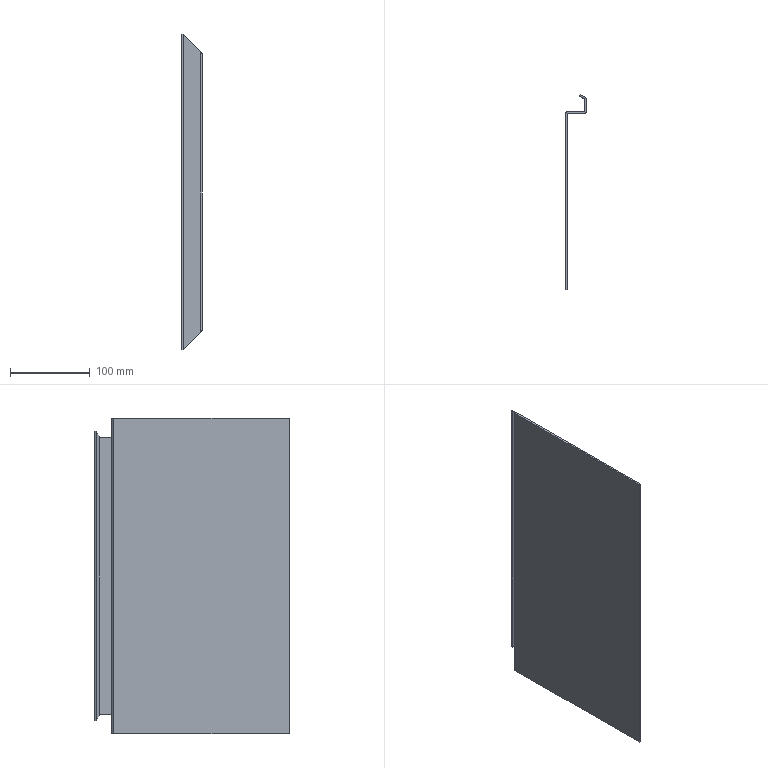Part | SolidWorks | features Cut 2, FlatPattern 1, SMBaseFlange 1, SheetMetal 1 | 1 solid | 32 faces | box 26 x 244.5 x 396 mm | volume 210973 mm3 | plane 22 | cylinder 6 | spline 4 | commonest cylinder face diameters 0.6 x3 4.6 x3
STEP:
#1=CARTESIAN_POINT('',(22.85,240.664,22.85));
#2=VERTEX_POINT('',#1);
#3=CARTESIAN_POINT('',(16.206,244.5,16.206));
#4=VERTEX_POINT('',#3);
#5=CARTESIAN_POINT('',(183.429,147.954,183.429));
#6=DIRECTION('',(-0.6547,0.378,-0.6547));
#7=VECTOR('',#6,1000.);
#8=LINE('',#5,#7);
#9=EDGE_CURVE('',#2,#4,#8,.T.);
#10=ORIENTED_EDGE('',*,*,#9,.T.);
#11=CARTESIAN_POINT('',(16.206,244.5,379.794));
#12=VERTEX_POINT('',#11);
#13=CARTESIAN_POINT('',(16.206,244.5,396.));
#14=DIRECTION('',(0.,0.,-1.));
#15=VECTOR('',#14,1000.);
#16=LINE('',#13,#15);
#17=EDGE_CURVE('',#12,#4,#16,.T.);
#18=ORIENTED_EDGE('',*,*,#17,.F.);
#19=CARTESIAN_POINT('',(22.85,240.664,373.15));
#20=VERTEX_POINT('',#19);
#21=CARTESIAN_POINT('',(13.714,245.938,382.286));
#22=DIRECTION('',(0.6547,-0.378,-0.6547));
#23=VECTOR('',#22,1000.);
#24=LINE('',#21,#23);
#25=EDGE_CURVE('',#12,#20,#24,.T.);
#26=ORIENTED_EDGE('',*,*,#25,.T.);
#27=CARTESIAN_POINT('',(22.85,240.664,396.));
#28=DIRECTION('',(0.,0.,-1.));
#29=VECTOR('',#28,1000.);
#30=LINE('',#27,#29);
#31=EDGE_CURVE('',#20,#2,#30,.T.);
#32=ORIENTED_EDGE('',*,*,#31,.T.);
#33=EDGE_LOOP('',(#10,#18,#26,#32));
#34=FACE_OUTER_BOUND('',#33,.T.);
#35=CARTESIAN_POINT('',(24.,240.,396.));
#36=DIRECTION('',(-0.5,-0.866,0.));
#37=DIRECTION('',(0.866,-0.5,0.));
#38=AXIS2_PLACEMENT_3D('',#35,#36,#37);
#39=PLANE('',#38);
#40=ADVANCED_FACE('',(#34),#39,.F.);
#41=ORIENTED_EDGE('',*,*,#17,.T.);
#42=CARTESIAN_POINT('',(15.206,242.768,16.206));
#43=VERTEX_POINT('',#42);
#44=CARTESIAN_POINT('',(16.206,244.5,16.206));
#45=DIRECTION('',(-0.5,-0.866,0.));
#46=VECTOR('',#45,1000.);
#47=LINE('',#44,#46);
#48=EDGE_CURVE('',#4,#43,#47,.T.);
#49=ORIENTED_EDGE('',*,*,#48,.T.);
#50=CARTESIAN_POINT('',(15.206,242.768,379.794));
#51=VERTEX_POINT('',#50);
#52=CARTESIAN_POINT('',(15.206,242.768,396.));
#53=DIRECTION('',(0.,0.,-1.));
#54=VECTOR('',#53,1000.);
#55=LINE('',#52,#54);
#56=EDGE_CURVE('',#51,#43,#55,.T.);
#57=ORIENTED_EDGE('',*,*,#56,.F.);
#58=CARTESIAN_POINT('',(16.206,244.5,379.794));
#59=DIRECTION('',(-0.5,-0.866,0.));
#60=VECTOR('',#59,1000.);
#61=LINE('',#58,#60);
#62=EDGE_CURVE('',#12,#51,#61,.T.);
#63=ORIENTED_EDGE('',*,*,#62,.F.);
#64=EDGE_LOOP('',(#41,#49,#57,#63));
#65=FACE_OUTER_BOUND('',#64,.T.);
#66=CARTESIAN_POINT('',(15.206,242.768,396.));
#67=DIRECTION('',(-0.866,0.5,0.));
#68=DIRECTION('',(-0.5,-0.866,0.));
#69=AXIS2_PLACEMENT_3D('',#66,#67,#68);
#70=PLANE('',#69);
#71=ADVANCED_FACE('',(#65),#70,.T.);
#72=ORIENTED_EDGE('',*,*,#56,.T.);
#73=CARTESIAN_POINT('',(21.85,238.932,22.85));
#74=VERTEX_POINT('',#73);
#75=CARTESIAN_POINT('',(182.429,146.222,183.429));
#76=DIRECTION('',(-0.6547,0.378,-0.6547));
#77=VECTOR('',#76,1000.);
#78=LINE('',#75,#77);
#79=EDGE_CURVE('',#74,#43,#78,.T.);
#80=ORIENTED_EDGE('',*,*,#79,.F.);
#81=CARTESIAN_POINT('',(21.85,238.932,373.15));
#82=VERTEX_POINT('',#81);
#83=CARTESIAN_POINT('',(21.85,238.932,396.));
#84=DIRECTION('',(0.,0.,-1.));
#85=VECTOR('',#84,1000.);
#86=LINE('',#83,#85);
#87=EDGE_CURVE('',#82,#74,#86,.T.);
#88=ORIENTED_EDGE('',*,*,#87,.F.);
#89=CARTESIAN_POINT('',(12.714,244.206,382.286));
#90=DIRECTION('',(0.6547,-0.378,-0.6547));
#91=VECTOR('',#90,1000.);
#92=LINE('',#89,#91);
#93=EDGE_CURVE('',#51,#82,#92,.T.);
#94=ORIENTED_EDGE('',*,*,#93,.F.);
#95=EDGE_LOOP('',(#72,#80,#88,#94));
#96=FACE_OUTER_BOUND('',#95,.T.);
#97=CARTESIAN_POINT('',(23.,238.268,396.));
#98=DIRECTION('',(-0.5,-0.866,0.));
#99=DIRECTION('',(0.866,-0.5,0.));
#100=AXIS2_PLACEMENT_3D('',#97,#98,#99);
#101=PLANE('',#100);
#102=ADVANCED_FACE('',(#96),#101,.T.);
#103=ORIENTED_EDGE('',*,*,#87,.T.);
#104=CARTESIAN_POINT('',(22.,238.672,24.));
#105=VERTEX_POINT('',#104);
#106=CARTESIAN_POINT('',(22.,238.672,24.));
#107=CARTESIAN_POINT('',(22.,238.782,24.));
#108=CARTESIAN_POINT('',(21.945,238.877,23.579));
#109=CARTESIAN_POINT('',(21.85,238.932,22.85));
#110=(BOUNDED_CURVE()B_SPLINE_CURVE(3,(#106,#107,#108,#109),.UNSPECIFIED.,.F.,.F.)B_SPLINE_CURVE_WITH_KNOTS((4,4),(3.142,4.189),.UNSPECIFIED.)CURVE()GEOMETRIC_REPRESENTATION_ITEM()RATIONAL_B_SPLINE_CURVE((1.,0.9107,0.9107,1.))REPRESENTATION_ITEM(''));
#111=EDGE_CURVE('',#105,#74,#110,.T.);
#112=ORIENTED_EDGE('',*,*,#111,.F.);
#113=CARTESIAN_POINT('',(22.,238.672,372.));
#114=VERTEX_POINT('',#113);
#115=CARTESIAN_POINT('',(22.,238.672,396.));
#116=DIRECTION('',(0.,0.,-1.));
#117=VECTOR('',#116,1000.);
#118=LINE('',#115,#117);
#119=EDGE_CURVE('',#114,#105,#118,.T.);
#120=ORIENTED_EDGE('',*,*,#119,.F.);
#121=CARTESIAN_POINT('',(21.85,238.932,373.15));
#122=CARTESIAN_POINT('',(21.945,238.877,372.421));
#123=CARTESIAN_POINT('',(22.,238.782,372.));
#124=CARTESIAN_POINT('',(22.,238.672,372.));
#125=(BOUNDED_CURVE()B_SPLINE_CURVE(3,(#121,#122,#123,#124),.UNSPECIFIED.,.F.,.F.)B_SPLINE_CURVE_WITH_KNOTS((4,4),(5.236,6.283),.UNSPECIFIED.)CURVE()GEOMETRIC_REPRESENTATION_ITEM()RATIONAL_B_SPLINE_CURVE((1.,0.9107,0.9107,1.))REPRESENTATION_ITEM(''));
#126=EDGE_CURVE('',#82,#114,#125,.T.);
#127=ORIENTED_EDGE('',*,*,#126,.F.);
#128=EDGE_LOOP('',(#103,#112,#120,#127));
#129=FACE_OUTER_BOUND('',#128,.T.);
#130=CARTESIAN_POINT('',(21.7,238.672,396.));
#131=DIRECTION('',(0.,0.,-1.));
#132=DIRECTION('',(-1.,0.,0.));
#133=AXIS2_PLACEMENT_3D('',#130,#131,#132);
#134=CYLINDRICAL_SURFACE('',#133,0.3);
#135=ADVANCED_FACE('',(#129),#134,.F.);
#136=ORIENTED_EDGE('',*,*,#119,.T.);
#137=CARTESIAN_POINT('',(22.,223.3,24.));
#138=VERTEX_POINT('',#137);
#139=CARTESIAN_POINT('',(22.,221.,24.));
#140=DIRECTION('',(0.,1.,0.));
#141=VECTOR('',#140,1000.);
#142=LINE('',#139,#141);
#143=EDGE_CURVE('',#138,#105,#142,.T.);
#144=ORIENTED_EDGE('',*,*,#143,.F.);
#145=CARTESIAN_POINT('',(22.,223.3,372.));
#146=VERTEX_POINT('',#145);
#147=CARTESIAN_POINT('',(22.,223.3,396.));
#148=DIRECTION('',(0.,0.,-1.));
#149=VECTOR('',#148,1000.);
#150=LINE('',#147,#149);
#151=EDGE_CURVE('',#146,#138,#150,.T.);
#152=ORIENTED_EDGE('',*,*,#151,.F.);
#153=CARTESIAN_POINT('',(22.,221.,372.));
#154=DIRECTION('',(0.,-1.,0.));
#155=VECTOR('',#154,1000.);
#156=LINE('',#153,#155);
#157=EDGE_CURVE('',#114,#146,#156,.T.);
#158=ORIENTED_EDGE('',*,*,#157,.F.);
#159=EDGE_LOOP('',(#136,#144,#152,#158));
#160=FACE_OUTER_BOUND('',#159,.T.);
#161=CARTESIAN_POINT('',(22.,221.,396.));
#162=DIRECTION('',(-1.,0.,0.));
#163=DIRECTION('',(0.,0.,1.));
#164=AXIS2_PLACEMENT_3D('',#161,#162,#163);
#165=PLANE('',#164);
#166=ADVANCED_FACE('',(#160),#165,.T.);
#167=ORIENTED_EDGE('',*,*,#151,.T.);
#168=CARTESIAN_POINT('',(21.7,223.,21.7));
#169=VERTEX_POINT('',#168);
#170=CARTESIAN_POINT('',(21.7,223.,21.7));
#171=CARTESIAN_POINT('',(21.876,223.,23.047));
#172=CARTESIAN_POINT('',(22.,223.124,24.));
#173=CARTESIAN_POINT('',(22.,223.3,24.));
#174=(BOUNDED_CURVE()B_SPLINE_CURVE(3,(#170,#171,#172,#173),.UNSPECIFIED.,.F.,.F.)B_SPLINE_CURVE_WITH_KNOTS((4,4),(1.571,3.142),.UNSPECIFIED.)CURVE()GEOMETRIC_REPRESENTATION_ITEM()RATIONAL_B_SPLINE_CURVE((1.,0.8047,0.8047,1.))REPRESENTATION_ITEM(''));
#175=EDGE_CURVE('',#169,#138,#174,.T.);
#176=ORIENTED_EDGE('',*,*,#175,.F.);
#177=CARTESIAN_POINT('',(21.7,223.,374.3));
#178=VERTEX_POINT('',#177);
#179=CARTESIAN_POINT('',(21.7,223.,396.));
#180=DIRECTION('',(0.,0.,-1.));
#181=VECTOR('',#180,1000.);
#182=LINE('',#179,#181);
#183=EDGE_CURVE('',#178,#169,#182,.T.);
#184=ORIENTED_EDGE('',*,*,#183,.F.);
#185=CARTESIAN_POINT('',(22.,223.3,372.));
#186=CARTESIAN_POINT('',(22.,223.124,372.));
#187=CARTESIAN_POINT('',(21.876,223.,372.953));
#188=CARTESIAN_POINT('',(21.7,223.,374.3));
#189=(BOUNDED_CURVE()B_SPLINE_CURVE(3,(#185,#186,#187,#188),.UNSPECIFIED.,.F.,.F.)B_SPLINE_CURVE_WITH_KNOTS((4,4),(0.,1.571),.UNSPECIFIED.)CURVE()GEOMETRIC_REPRESENTATION_ITEM()RATIONAL_B_SPLINE_CURVE((1.,0.8047,0.8047,1.))REPRESENTATION_ITEM(''));
#190=EDGE_CURVE('',#146,#178,#189,.T.);
#191=ORIENTED_EDGE('',*,*,#190,.F.);
#192=EDGE_LOOP('',(#167,#176,#184,#191));
#193=FACE_OUTER_BOUND('',#192,.T.);
#194=CARTESIAN_POINT('',(21.7,223.3,396.));
#195=DIRECTION('',(0.,0.,-1.));
#196=DIRECTION('',(-1.,0.,0.));
#197=AXIS2_PLACEMENT_3D('',#194,#195,#196);
#198=CYLINDRICAL_SURFACE('',#197,0.3);
#199=ADVANCED_FACE('',(#193),#198,.F.);
#200=ORIENTED_EDGE('',*,*,#183,.T.);
#201=CARTESIAN_POINT('',(0.3,223.,0.3));
#202=VERTEX_POINT('',#201);
#203=CARTESIAN_POINT('',(198.,223.,198.));
#204=DIRECTION('',(0.7071,0.,0.7071));
#205=VECTOR('',#204,1000.);
#206=LINE('',#203,#205);
#207=EDGE_CURVE('',#202,#169,#206,.T.);
#208=ORIENTED_EDGE('',*,*,#207,.F.);
#209=CARTESIAN_POINT('',(0.3,223.,395.7));
#210=VERTEX_POINT('',#209);
#211=CARTESIAN_POINT('',(0.3,223.,396.));
#212=DIRECTION('',(0.,0.,-1.));
#213=VECTOR('',#212,1000.);
#214=LINE('',#211,#213);
#215=EDGE_CURVE('',#210,#202,#214,.T.);
#216=ORIENTED_EDGE('',*,*,#215,.F.);
#217=CARTESIAN_POINT('',(0.,223.,396.));
#218=DIRECTION('',(-0.7071,0.,0.7071));
#219=VECTOR('',#218,1000.);
#220=LINE('',#217,#219);
#221=EDGE_CURVE('',#178,#210,#220,.T.);
#222=ORIENTED_EDGE('',*,*,#221,.F.);
#223=EDGE_LOOP('',(#200,#208,#216,#222));
#224=FACE_OUTER_BOUND('',#223,.T.);
#225=CARTESIAN_POINT('',(0.,223.,396.));
#226=DIRECTION('',(0.,1.,0.));
#227=DIRECTION('',(0.,0.,1.));
#228=AXIS2_PLACEMENT_3D('',#225,#226,#227);
#229=PLANE('',#228);
#230=ADVANCED_FACE('',(#224),#229,.T.);
#231=CARTESIAN_POINT('',(0.3,221.,0.3));
#232=VERTEX_POINT('',#231);
#233=CARTESIAN_POINT('',(21.7,221.,21.7));
#234=VERTEX_POINT('',#233);
#235=CARTESIAN_POINT('',(198.,221.,198.));
#236=DIRECTION('',(0.7071,0.,0.7071));
#237=VECTOR('',#236,1000.);
#238=LINE('',#235,#237);
#239=EDGE_CURVE('',#232,#234,#238,.T.);
#240=ORIENTED_EDGE('',*,*,#239,.T.);
#241=CARTESIAN_POINT('',(21.7,221.,374.3));
#242=VERTEX_POINT('',#241);
#243=CARTESIAN_POINT('',(21.7,221.,396.));
#244=DIRECTION('',(0.,0.,-1.));
#245=VECTOR('',#244,1000.);
#246=LINE('',#243,#245);
#247=EDGE_CURVE('',#242,#234,#246,.T.);
#248=ORIENTED_EDGE('',*,*,#247,.F.);
#249=CARTESIAN_POINT('',(0.3,221.,395.7));
#250=VERTEX_POINT('',#249);
#251=CARTESIAN_POINT('',(0.,221.,396.));
#252=DIRECTION('',(-0.7071,0.,0.7071));
#253=VECTOR('',#252,1000.);
#254=LINE('',#251,#253);
#255=EDGE_CURVE('',#242,#250,#254,.T.);
#256=ORIENTED_EDGE('',*,*,#255,.T.);
#257=CARTESIAN_POINT('',(0.3,221.,396.));
#258=DIRECTION('',(0.,0.,-1.));
#259=VECTOR('',#258,1000.);
#260=LINE('',#257,#259);
#261=EDGE_CURVE('',#250,#232,#260,.T.);
#262=ORIENTED_EDGE('',*,*,#261,.T.);
#263=EDGE_LOOP('',(#240,#248,#256,#262));
#264=FACE_OUTER_BOUND('',#263,.T.);
#265=CARTESIAN_POINT('',(0.,221.,396.));
#266=DIRECTION('',(0.,1.,0.));
#267=DIRECTION('',(0.,0.,1.));
#268=AXIS2_PLACEMENT_3D('',#265,#266,#267);
#269=PLANE('',#268);
#270=ADVANCED_FACE('',(#264),#269,.F.);
#271=CARTESIAN_POINT('',(24.,223.3,24.));
#272=VERTEX_POINT('',#271);
#273=CARTESIAN_POINT('',(21.7,221.,21.7));
#274=CARTESIAN_POINT('',(23.047,221.,23.047));
#275=CARTESIAN_POINT('',(24.,221.953,24.));
#276=CARTESIAN_POINT('',(24.,223.3,24.));
#277=(BOUNDED_CURVE()B_SPLINE_CURVE(3,(#273,#274,#275,#276),.UNSPECIFIED.,.F.,.F.)B_SPLINE_CURVE_WITH_KNOTS((4,4),(1.571,3.142),.UNSPECIFIED.)CURVE()GEOMETRIC_REPRESENTATION_ITEM()RATIONAL_B_SPLINE_CURVE((1.,0.8047,0.8047,1.))REPRESENTATION_ITEM(''));
#278=EDGE_CURVE('',#234,#272,#277,.T.);
#279=ORIENTED_EDGE('',*,*,#278,.T.);
#280=CARTESIAN_POINT('',(24.,223.3,372.));
#281=VERTEX_POINT('',#280);
#282=CARTESIAN_POINT('',(24.,223.3,396.));
#283=DIRECTION('',(0.,0.,-1.));
#284=VECTOR('',#283,1000.);
#285=LINE('',#282,#284);
#286=EDGE_CURVE('',#281,#272,#285,.T.);
#287=ORIENTED_EDGE('',*,*,#286,.F.);
#288=CARTESIAN_POINT('',(24.,223.3,372.));
#289=CARTESIAN_POINT('',(24.,221.953,372.));
#290=CARTESIAN_POINT('',(23.047,221.,372.953));
#291=CARTESIAN_POINT('',(21.7,221.,374.3));
#292=(BOUNDED_CURVE()B_SPLINE_CURVE(3,(#288,#289,#290,#291),.UNSPECIFIED.,.F.,.F.)B_SPLINE_CURVE_WITH_KNOTS((4,4),(0.,1.571),.UNSPECIFIED.)CURVE()GEOMETRIC_REPRESENTATION_ITEM()RATIONAL_B_SPLINE_CURVE((1.,0.8047,0.8047,1.))REPRESENTATION_ITEM(''));
#293=EDGE_CURVE('',#281,#242,#292,.T.);
#294=ORIENTED_EDGE('',*,*,#293,.T.);
#295=ORIENTED_EDGE('',*,*,#247,.T.);
#296=EDGE_LOOP('',(#279,#287,#294,#295));
#297=FACE_OUTER_BOUND('',#296,.T.);
#298=CARTESIAN_POINT('',(21.7,223.3,396.));
#299=DIRECTION('',(0.,0.,-1.));
#300=DIRECTION('',(-1.,0.,0.));
#301=AXIS2_PLACEMENT_3D('',#298,#299,#300);
#302=CYLINDRICAL_SURFACE('',#301,2.3);
#303=ADVANCED_FACE('',(#297),#302,.T.);
#304=CARTESIAN_POINT('',(24.,238.672,24.));
#305=VERTEX_POINT('',#304);
#306=CARTESIAN_POINT('',(24.,221.,24.));
#307=DIRECTION('',(0.,1.,0.));
#308=VECTOR('',#307,1000.);
#309=LINE('',#306,#308);
#310=EDGE_CURVE('',#272,#305,#309,.T.);
#311=ORIENTED_EDGE('',*,*,#310,.T.);
#312=CARTESIAN_POINT('',(24.,238.672,372.));
#313=VERTEX_POINT('',#312);
#314=CARTESIAN_POINT('',(24.,238.672,396.));
#315=DIRECTION('',(0.,0.,-1.));
#316=VECTOR('',#315,1000.);
#317=LINE('',#314,#316);
#318=EDGE_CURVE('',#313,#305,#317,.T.);
#319=ORIENTED_EDGE('',*,*,#318,.F.);
#320=CARTESIAN_POINT('',(24.,221.,372.));
#321=DIRECTION('',(0.,-1.,0.));
#322=VECTOR('',#321,1000.);
#323=LINE('',#320,#322);
#324=EDGE_CURVE('',#313,#281,#323,.T.);
#325=ORIENTED_EDGE('',*,*,#324,.T.);
#326=ORIENTED_EDGE('',*,*,#286,.T.);
#327=EDGE_LOOP('',(#311,#319,#325,#326));
#328=FACE_OUTER_BOUND('',#327,.T.);
#329=CARTESIAN_POINT('',(24.,221.,396.));
#330=DIRECTION('',(-1.,0.,0.));
#331=DIRECTION('',(0.,0.,1.));
#332=AXIS2_PLACEMENT_3D('',#329,#330,#331);
#333=PLANE('',#332);
#334=ADVANCED_FACE('',(#328),#333,.F.);
#335=CARTESIAN_POINT('',(24.,238.672,24.));
#336=CARTESIAN_POINT('',(24.,239.514,24.));
#337=CARTESIAN_POINT('',(23.579,240.243,23.579));
#338=CARTESIAN_POINT('',(22.85,240.664,22.85));
#339=(BOUNDED_CURVE()B_SPLINE_CURVE(3,(#335,#336,#337,#338),.UNSPECIFIED.,.F.,.F.)B_SPLINE_CURVE_WITH_KNOTS((4,4),(3.142,4.189),.UNSPECIFIED.)CURVE()GEOMETRIC_REPRESENTATION_ITEM()RATIONAL_B_SPLINE_CURVE((1.,0.9107,0.9107,1.))REPRESENTATION_ITEM(''));
#340=EDGE_CURVE('',#305,#2,#339,.T.);
#341=ORIENTED_EDGE('',*,*,#340,.T.);
#342=ORIENTED_EDGE('',*,*,#31,.F.);
#343=CARTESIAN_POINT('',(22.85,240.664,373.15));
#344=CARTESIAN_POINT('',(23.579,240.243,372.421));
#345=CARTESIAN_POINT('',(24.,239.514,372.));
#346=CARTESIAN_POINT('',(24.,238.672,372.));
#347=(BOUNDED_CURVE()B_SPLINE_CURVE(3,(#343,#344,#345,#346),.UNSPECIFIED.,.F.,.F.)B_SPLINE_CURVE_WITH_KNOTS((4,4),(5.236,6.283),.UNSPECIFIED.)CURVE()GEOMETRIC_REPRESENTATION_ITEM()RATIONAL_B_SPLINE_CURVE((1.,0.9107,0.9107,1.))REPRESENTATION_ITEM(''));
#348=EDGE_CURVE('',#20,#313,#347,.T.);
#349=ORIENTED_EDGE('',*,*,#348,.T.);
#350=ORIENTED_EDGE('',*,*,#318,.T.);
#351=EDGE_LOOP('',(#341,#342,#349,#350));
#352=FACE_OUTER_BOUND('',#351,.T.);
#353=CARTESIAN_POINT('',(21.7,238.672,396.));
#354=DIRECTION('',(0.,0.,-1.));
#355=DIRECTION('',(-1.,0.,0.));
#356=AXIS2_PLACEMENT_3D('',#353,#354,#355);
#357=CYLINDRICAL_SURFACE('',#356,2.3);
#358=ADVANCED_FACE('',(#352),#357,.T.);
#359=CARTESIAN_POINT('',(0.,220.7,396.));
#360=VERTEX_POINT('',#359);
#361=CARTESIAN_POINT('',(-2.,220.7,396.));
#362=VERTEX_POINT('',#361);
#363=CARTESIAN_POINT('',(0.,220.7,396.));
#364=DIRECTION('',(-1.,0.,0.));
#365=VECTOR('',#364,1000.);
#366=LINE('',#363,#365);
#367=EDGE_CURVE('',#360,#362,#366,.T.);
#368=ORIENTED_EDGE('',*,*,#367,.F.);
#369=CARTESIAN_POINT('',(0.3,221.,396.));
#370=VERTEX_POINT('',#369);
#371=CARTESIAN_POINT('',(0.3,220.7,396.));
#372=DIRECTION('',(0.,0.,-1.));
#373=DIRECTION('',(1.,0.,0.));
#374=AXIS2_PLACEMENT_3D('',#371,#372,#373);
#375=CIRCLE('',#374,0.3);
#376=EDGE_CURVE('',#360,#370,#375,.T.);
#377=ORIENTED_EDGE('',*,*,#376,.T.);
#378=CARTESIAN_POINT('',(0.3,223.,396.));
#379=VERTEX_POINT('',#378);
#380=CARTESIAN_POINT('',(0.3,223.,396.));
#381=DIRECTION('',(0.,-1.,0.));
#382=VECTOR('',#381,1000.);
#383=LINE('',#380,#382);
#384=EDGE_CURVE('',#379,#370,#383,.T.);
#385=ORIENTED_EDGE('',*,*,#384,.F.);
#386=CARTESIAN_POINT('',(0.3,220.7,396.));
#387=DIRECTION('',(0.,0.,-1.));
#388=DIRECTION('',(1.,0.,0.));
#389=AXIS2_PLACEMENT_3D('',#386,#387,#388);
#390=CIRCLE('',#389,2.3);
#391=EDGE_CURVE('',#362,#379,#390,.T.);
#392=ORIENTED_EDGE('',*,*,#391,.F.);
#393=EDGE_LOOP('',(#368,#377,#385,#392));
#394=FACE_OUTER_BOUND('',#393,.T.);
#395=CARTESIAN_POINT('',(0.,220.7,396.));
#396=DIRECTION('',(0.,0.,1.));
#397=DIRECTION('',(1.,0.,0.));
#398=AXIS2_PLACEMENT_3D('',#395,#396,#397);
#399=PLANE('',#398);
#400=ADVANCED_FACE('',(#394),#399,.T.);
#401=CARTESIAN_POINT('',(0.,0.,396.));
#402=VERTEX_POINT('',#401);
#403=CARTESIAN_POINT('',(0.,0.,396.));
#404=DIRECTION('',(0.,1.,0.));
#405=VECTOR('',#404,1000.);
#406=LINE('',#403,#405);
#407=EDGE_CURVE('',#402,#360,#406,.T.);
#408=ORIENTED_EDGE('',*,*,#407,.T.);
#409=ORIENTED_EDGE('',*,*,#367,.T.);
#410=CARTESIAN_POINT('',(-2.,0.,396.));
#411=VERTEX_POINT('',#410);
#412=CARTESIAN_POINT('',(-2.,0.,396.));
#413=DIRECTION('',(0.,1.,0.));
#414=VECTOR('',#413,1000.);
#415=LINE('',#412,#414);
#416=EDGE_CURVE('',#411,#362,#415,.T.);
#417=ORIENTED_EDGE('',*,*,#416,.F.);
#418=CARTESIAN_POINT('',(0.,0.,396.));
#419=DIRECTION('',(-1.,0.,0.));
#420=VECTOR('',#419,1000.);
#421=LINE('',#418,#420);
#422=EDGE_CURVE('',#402,#411,#421,.T.);
#423=ORIENTED_EDGE('',*,*,#422,.F.);
#424=EDGE_LOOP('',(#408,#409,#417,#423));
#425=FACE_OUTER_BOUND('',#424,.T.);
#426=CARTESIAN_POINT('',(0.3,223.,396.));
#427=DIRECTION('',(0.,0.,1.));
#428=DIRECTION('',(1.,0.,0.));
#429=AXIS2_PLACEMENT_3D('',#426,#427,#428);
#430=PLANE('',#429);
#431=ADVANCED_FACE('',(#425),#430,.T.);
#432=CARTESIAN_POINT('',(0.3,221.,0.));
#433=VERTEX_POINT('',#432);
#434=CARTESIAN_POINT('',(0.3,223.,0.));
#435=VERTEX_POINT('',#434);
#436=CARTESIAN_POINT('',(0.3,221.,0.));
#437=DIRECTION('',(0.,1.,0.));
#438=VECTOR('',#437,1000.);
#439=LINE('',#436,#438);
#440=EDGE_CURVE('',#433,#435,#439,.T.);
#441=ORIENTED_EDGE('',*,*,#440,.F.);
#442=CARTESIAN_POINT('',(0.,220.7,0.));
#443=VERTEX_POINT('',#442);
#444=CARTESIAN_POINT('',(0.3,220.7,0.));
#445=DIRECTION('',(0.,0.,-1.));
#446=DIRECTION('',(1.,0.,0.));
#447=AXIS2_PLACEMENT_3D('',#444,#445,#446);
#448=CIRCLE('',#447,0.3);
#449=EDGE_CURVE('',#443,#433,#448,.T.);
#450=ORIENTED_EDGE('',*,*,#449,.F.);
#451=CARTESIAN_POINT('',(-2.,220.7,0.));
#452=VERTEX_POINT('',#451);
#453=CARTESIAN_POINT('',(-2.,220.7,0.));
#454=DIRECTION('',(1.,0.,0.));
#455=VECTOR('',#454,1000.);
#456=LINE('',#453,#455);
#457=EDGE_CURVE('',#452,#443,#456,.T.);
#458=ORIENTED_EDGE('',*,*,#457,.F.);
#459=CARTESIAN_POINT('',(0.3,220.7,0.));
#460=DIRECTION('',(0.,0.,-1.));
#461=DIRECTION('',(1.,0.,0.));
#462=AXIS2_PLACEMENT_3D('',#459,#460,#461);
#463=CIRCLE('',#462,2.3);
#464=EDGE_CURVE('',#452,#435,#463,.T.);
#465=ORIENTED_EDGE('',*,*,#464,.T.);
#466=EDGE_LOOP('',(#441,#450,#458,#465));
#467=FACE_OUTER_BOUND('',#466,.T.);
#468=CARTESIAN_POINT('',(0.3,221.,0.));
#469=DIRECTION('',(0.,0.,-1.));
#470=DIRECTION('',(-1.,0.,0.));
#471=AXIS2_PLACEMENT_3D('',#468,#469,#470);
#472=PLANE('',#471);
#473=ADVANCED_FACE('',(#467),#472,.T.);
#474=ORIENTED_EDGE('',*,*,#464,.F.);
#475=CARTESIAN_POINT('',(-2.,220.7,396.));
#476=DIRECTION('',(0.,0.,-1.));
#477=VECTOR('',#476,1000.);
#478=LINE('',#475,#477);
#479=EDGE_CURVE('',#362,#452,#478,.T.);
#480=ORIENTED_EDGE('',*,*,#479,.F.);
#481=ORIENTED_EDGE('',*,*,#391,.T.);
#482=CARTESIAN_POINT('',(0.3,223.,396.));
#483=DIRECTION('',(0.,0.,-1.));
#484=VECTOR('',#483,1000.);
#485=LINE('',#482,#484);
#486=EDGE_CURVE('',#379,#210,#485,.T.);
#487=ORIENTED_EDGE('',*,*,#486,.T.);
#488=ORIENTED_EDGE('',*,*,#215,.T.);
#489=CARTESIAN_POINT('',(0.3,223.,396.));
#490=DIRECTION('',(0.,0.,1.));
#491=VECTOR('',#490,1000.);
#492=LINE('',#489,#491);
#493=EDGE_CURVE('',#435,#202,#492,.T.);
#494=ORIENTED_EDGE('',*,*,#493,.F.);
#495=EDGE_LOOP('',(#474,#480,#481,#487,#488,#494));
#496=FACE_OUTER_BOUND('',#495,.T.);
#497=CARTESIAN_POINT('',(0.3,220.7,396.));
#498=DIRECTION('',(0.,0.,-1.));
#499=DIRECTION('',(-1.,0.,0.));
#500=AXIS2_PLACEMENT_3D('',#497,#498,#499);
#501=CYLINDRICAL_SURFACE('',#500,2.3);
#502=ADVANCED_FACE('',(#496),#501,.T.);
#503=CARTESIAN_POINT('',(-2.,0.,0.));
#504=VERTEX_POINT('',#503);
#505=CARTESIAN_POINT('',(-2.,0.,0.));
#506=DIRECTION('',(0.,1.,0.));
#507=VECTOR('',#506,1000.);
#508=LINE('',#505,#507);
#509=EDGE_CURVE('',#504,#452,#508,.T.);
#510=ORIENTED_EDGE('',*,*,#509,.F.);
#511=CARTESIAN_POINT('',(-2.,0.,396.));
#512=DIRECTION('',(0.,0.,-1.));
#513=VECTOR('',#512,1000.);
#514=LINE('',#511,#513);
#515=EDGE_CURVE('',#411,#504,#514,.T.);
#516=ORIENTED_EDGE('',*,*,#515,.F.);
#517=ORIENTED_EDGE('',*,*,#416,.T.);
#518=ORIENTED_EDGE('',*,*,#479,.T.);
#519=EDGE_LOOP('',(#510,#516,#517,#518));
#520=FACE_OUTER_BOUND('',#519,.T.);
#521=CARTESIAN_POINT('',(-2.,0.,396.));
#522=DIRECTION('',(-1.,0.,0.));
#523=DIRECTION('',(0.,0.,1.));
#524=AXIS2_PLACEMENT_3D('',#521,#522,#523);
#525=PLANE('',#524);
#526=ADVANCED_FACE('',(#520),#525,.T.);
#527=CARTESIAN_POINT('',(0.,0.,0.));
#528=VERTEX_POINT('',#527);
#529=CARTESIAN_POINT('',(0.,0.,0.));
#530=DIRECTION('',(-1.,0.,0.));
#531=VECTOR('',#530,1000.);
#532=LINE('',#529,#531);
#533=EDGE_CURVE('',#528,#504,#532,.T.);
#534=ORIENTED_EDGE('',*,*,#533,.F.);
#535=CARTESIAN_POINT('',(0.,0.,396.));
#536=DIRECTION('',(0.,0.,-1.));
#537=VECTOR('',#536,1000.);
#538=LINE('',#535,#537);
#539=EDGE_CURVE('',#402,#528,#538,.T.);
#540=ORIENTED_EDGE('',*,*,#539,.F.);
#541=ORIENTED_EDGE('',*,*,#422,.T.);
#542=ORIENTED_EDGE('',*,*,#515,.T.);
#543=EDGE_LOOP('',(#534,#540,#541,#542));
#544=FACE_OUTER_BOUND('',#543,.T.);
#545=CARTESIAN_POINT('',(0.,0.,396.));
#546=DIRECTION('',(0.,-1.,0.));
#547=DIRECTION('',(0.,0.,-1.));
#548=AXIS2_PLACEMENT_3D('',#545,#546,#547);
#549=PLANE('',#548);
#550=ADVANCED_FACE('',(#544),#549,.T.);
#551=CARTESIAN_POINT('',(0.,0.,0.));
#552=DIRECTION('',(0.,1.,0.));
#553=VECTOR('',#552,1000.);
#554=LINE('',#551,#553);
#555=EDGE_CURVE('',#528,#443,#554,.T.);
#556=ORIENTED_EDGE('',*,*,#555,.T.);
#557=CARTESIAN_POINT('',(0.,220.7,396.));
#558=DIRECTION('',(0.,0.,-1.));
#559=VECTOR('',#558,1000.);
#560=LINE('',#557,#559);
#561=EDGE_CURVE('',#360,#443,#560,.T.);
#562=ORIENTED_EDGE('',*,*,#561,.F.);
#563=ORIENTED_EDGE('',*,*,#407,.F.);
#564=ORIENTED_EDGE('',*,*,#539,.T.);
#565=EDGE_LOOP('',(#556,#562,#563,#564));
#566=FACE_OUTER_BOUND('',#565,.T.);
#567=CARTESIAN_POINT('',(0.,0.,396.));
#568=DIRECTION('',(-1.,0.,0.));
#569=DIRECTION('',(0.,0.,1.));
#570=AXIS2_PLACEMENT_3D('',#567,#568,#569);
#571=PLANE('',#570);
#572=ADVANCED_FACE('',(#566),#571,.F.);
#573=ORIENTED_EDGE('',*,*,#449,.T.);
#574=CARTESIAN_POINT('',(0.3,221.,396.));
#575=DIRECTION('',(0.,0.,1.));
#576=VECTOR('',#575,1000.);
#577=LINE('',#574,#576);
#578=EDGE_CURVE('',#433,#232,#577,.T.);
#579=ORIENTED_EDGE('',*,*,#578,.T.);
#580=ORIENTED_EDGE('',*,*,#261,.F.);
#581=CARTESIAN_POINT('',(0.3,221.,396.));
#582=DIRECTION('',(0.,0.,-1.));
#583=VECTOR('',#582,1000.);
#584=LINE('',#581,#583);
#585=EDGE_CURVE('',#370,#250,#584,.T.);
#586=ORIENTED_EDGE('',*,*,#585,.F.);
#587=ORIENTED_EDGE('',*,*,#376,.F.);
#588=ORIENTED_EDGE('',*,*,#561,.T.);
#589=EDGE_LOOP('',(#573,#579,#580,#586,#587,#588));
#590=FACE_OUTER_BOUND('',#589,.T.);
#591=CARTESIAN_POINT('',(0.3,220.7,396.));
#592=DIRECTION('',(0.,0.,-1.));
#593=DIRECTION('',(-1.,0.,0.));
#594=AXIS2_PLACEMENT_3D('',#591,#592,#593);
#595=CYLINDRICAL_SURFACE('',#594,0.3);
#596=ADVANCED_FACE('',(#590),#595,.F.);
#597=ORIENTED_EDGE('',*,*,#509,.T.);
#598=ORIENTED_EDGE('',*,*,#457,.T.);
#599=ORIENTED_EDGE('',*,*,#555,.F.);
#600=ORIENTED_EDGE('',*,*,#533,.T.);
#601=EDGE_LOOP('',(#597,#598,#599,#600));
#602=FACE_OUTER_BOUND('',#601,.T.);
#603=CARTESIAN_POINT('',(21.7,238.672,0.));
#604=DIRECTION('',(0.,0.,1.));
#605=DIRECTION('',(1.,0.,0.));
#606=AXIS2_PLACEMENT_3D('',#603,#604,#605);
#607=PLANE('',#606);
#608=ADVANCED_FACE('',(#602),#607,.F.);
#609=CARTESIAN_POINT('',(0.3,223.,395.7));
#610=DIRECTION('',(0.,-1.,0.));
#611=VECTOR('',#610,1000.);
#612=LINE('',#609,#611);
#613=EDGE_CURVE('',#210,#250,#612,.T.);
#614=ORIENTED_EDGE('',*,*,#613,.F.);
#615=ORIENTED_EDGE('',*,*,#486,.F.);
#616=ORIENTED_EDGE('',*,*,#384,.T.);
#617=ORIENTED_EDGE('',*,*,#585,.T.);
#618=EDGE_LOOP('',(#614,#615,#616,#617));
#619=FACE_OUTER_BOUND('',#618,.T.);
#620=CARTESIAN_POINT('',(0.3,223.,396.));
#621=DIRECTION('',(1.,0.,0.));
#622=DIRECTION('',(0.,0.,-1.));
#623=AXIS2_PLACEMENT_3D('',#620,#621,#622);
#624=PLANE('',#623);
#625=ADVANCED_FACE('',(#619),#624,.T.);
#626=ORIENTED_EDGE('',*,*,#221,.T.);
#627=ORIENTED_EDGE('',*,*,#613,.T.);
#628=ORIENTED_EDGE('',*,*,#255,.F.);
#629=CARTESIAN_POINT('',(21.7,223.,374.3));
#630=DIRECTION('',(0.,-1.,0.));
#631=VECTOR('',#630,1000.);
#632=LINE('',#629,#631);
#633=EDGE_CURVE('',#178,#242,#632,.T.);
#634=ORIENTED_EDGE('',*,*,#633,.F.);
#635=EDGE_LOOP('',(#626,#627,#628,#634));
#636=FACE_OUTER_BOUND('',#635,.T.);
#637=CARTESIAN_POINT('',(0.,223.,396.));
#638=DIRECTION('',(-0.7071,0.,-0.7071));
#639=DIRECTION('',(-0.7071,0.,0.7071));
#640=AXIS2_PLACEMENT_3D('',#637,#638,#639);
#641=PLANE('',#640);
#642=ADVANCED_FACE('',(#636),#641,.F.);
#643=CARTESIAN_POINT('',(24.,223.3,372.));
#644=DIRECTION('',(-1.,0.,0.));
#645=VECTOR('',#644,1000.);
#646=LINE('',#643,#645);
#647=EDGE_CURVE('',#281,#146,#646,.T.);
#648=ORIENTED_EDGE('',*,*,#647,.F.);
#649=ORIENTED_EDGE('',*,*,#324,.F.);
#650=CARTESIAN_POINT('',(24.,238.672,372.));
#651=DIRECTION('',(-1.,0.,0.));
#652=VECTOR('',#651,1000.);
#653=LINE('',#650,#652);
#654=EDGE_CURVE('',#313,#114,#653,.T.);
#655=ORIENTED_EDGE('',*,*,#654,.T.);
#656=ORIENTED_EDGE('',*,*,#157,.T.);
#657=EDGE_LOOP('',(#648,#649,#655,#656));
#658=FACE_OUTER_BOUND('',#657,.T.);
#659=CARTESIAN_POINT('',(24.,221.,372.));
#660=DIRECTION('',(0.,0.,-1.));
#661=DIRECTION('',(0.,-1.,0.));
#662=AXIS2_PLACEMENT_3D('',#659,#660,#661);
#663=PLANE('',#662);
#664=ADVANCED_FACE('',(#658),#663,.F.);
#665=CARTESIAN_POINT('',(22.85,240.664,373.15));
#666=DIRECTION('',(-0.5,-0.866,0.));
#667=VECTOR('',#666,1000.);
#668=LINE('',#665,#667);
#669=EDGE_CURVE('',#20,#82,#668,.T.);
#670=ORIENTED_EDGE('',*,*,#669,.F.);
#671=ORIENTED_EDGE('',*,*,#25,.F.);
#672=ORIENTED_EDGE('',*,*,#62,.T.);
#673=ORIENTED_EDGE('',*,*,#93,.T.);
#674=EDGE_LOOP('',(#670,#671,#672,#673));
#675=FACE_OUTER_BOUND('',#674,.T.);
#676=CARTESIAN_POINT('',(13.714,245.938,382.286));
#677=DIRECTION('',(-0.5669,0.3273,-0.7559));
#678=DIRECTION('',(0.6547,-0.378,-0.6547));
#679=AXIS2_PLACEMENT_3D('',#676,#677,#678);
#680=PLANE('',#679);
#681=ADVANCED_FACE('',(#675),#680,.F.);
#682=ORIENTED_EDGE('',*,*,#654,.F.);
#683=ORIENTED_EDGE('',*,*,#348,.F.);
#684=ORIENTED_EDGE('',*,*,#669,.T.);
#685=ORIENTED_EDGE('',*,*,#126,.T.);
#686=EDGE_LOOP('',(#682,#683,#684,#685));
#687=FACE_OUTER_BOUND('',#686,.T.);
#688=CARTESIAN_POINT('',(22.,238.672,372.));
#689=CARTESIAN_POINT('',(22.667,238.672,372.));
#690=CARTESIAN_POINT('',(23.333,238.672,372.));
#691=CARTESIAN_POINT('',(24.,238.672,372.));
#692=CARTESIAN_POINT('',(22.,238.072,372.));
#693=CARTESIAN_POINT('',(22.667,236.739,372.));
#694=CARTESIAN_POINT('',(23.333,235.405,372.));
#695=CARTESIAN_POINT('',(24.,234.072,372.));
#696=CARTESIAN_POINT('',(21.4,238.072,376.6));
#697=CARTESIAN_POINT('',(20.733,236.739,376.6));
#698=CARTESIAN_POINT('',(20.067,235.405,376.6));
#699=CARTESIAN_POINT('',(19.4,234.072,376.6));
#700=CARTESIAN_POINT('',(21.4,238.672,376.6));
#701=CARTESIAN_POINT('',(20.733,238.672,376.6));
#702=CARTESIAN_POINT('',(20.067,238.672,376.6));
#703=CARTESIAN_POINT('',(19.4,238.672,376.6));
#704=CARTESIAN_POINT('',(21.4,239.272,376.6));
#705=CARTESIAN_POINT('',(20.733,240.605,376.6));
#706=CARTESIAN_POINT('',(20.067,241.939,376.6));
#707=CARTESIAN_POINT('',(19.4,243.272,376.6));
#708=CARTESIAN_POINT('',(22.,239.272,372.));
#709=CARTESIAN_POINT('',(22.667,240.605,372.));
#710=CARTESIAN_POINT('',(23.333,241.939,372.));
#711=CARTESIAN_POINT('',(24.,243.272,372.));
#712=CARTESIAN_POINT('',(22.,238.672,372.));
#713=CARTESIAN_POINT('',(22.667,238.672,372.));
#714=CARTESIAN_POINT('',(23.333,238.672,372.));
#715=CARTESIAN_POINT('',(24.,238.672,372.));
#716=(BOUNDED_SURFACE()B_SPLINE_SURFACE(3,3,((#688,#689,#690,#691),(#692,#693,#694,#695),(#696,#697,#698,#699),(#700,#701,#702,#703),(#704,#705,#706,#707),(#708,#709,#710,#711),(#712,#713,#714,#715)),.UNSPECIFIED.,.T.,.F.,.F.)B_SPLINE_SURFACE_WITH_KNOTS((4,3,4),(4,4),(0.,0.5,1.),(0.,1.),.UNSPECIFIED.)GEOMETRIC_REPRESENTATION_ITEM()RATIONAL_B_SPLINE_SURFACE(((1.,1.,1.,1.),(0.3333,0.3333,0.3333,0.3333),(0.3333,0.3333,0.3333,0.3333),(1.,1.,1.,1.),(0.3333,0.3333,0.3333,0.3333),(0.3333,0.3333,0.3333,0.3333),(1.,1.,1.,1.)))REPRESENTATION_ITEM('')SURFACE());
#717=ADVANCED_FACE('',(#687),#716,.T.);
#718=ORIENTED_EDGE('',*,*,#633,.T.);
#719=ORIENTED_EDGE('',*,*,#293,.F.);
#720=ORIENTED_EDGE('',*,*,#647,.T.);
#721=ORIENTED_EDGE('',*,*,#190,.T.);
#722=EDGE_LOOP('',(#718,#719,#720,#721));
#723=FACE_OUTER_BOUND('',#722,.T.);
#724=CARTESIAN_POINT('',(22.,223.3,372.));
#725=CARTESIAN_POINT('',(22.667,223.3,372.));
#726=CARTESIAN_POINT('',(23.333,223.3,372.));
#727=CARTESIAN_POINT('',(24.,223.3,372.));
#728=CARTESIAN_POINT('',(22.,222.7,372.));
#729=CARTESIAN_POINT('',(22.667,221.367,372.));
#730=CARTESIAN_POINT('',(23.333,220.033,372.));
#731=CARTESIAN_POINT('',(24.,218.7,372.));
#732=CARTESIAN_POINT('',(21.4,222.7,376.6));
#733=CARTESIAN_POINT('',(20.733,221.367,376.6));
#734=CARTESIAN_POINT('',(20.067,220.033,376.6));
#735=CARTESIAN_POINT('',(19.4,218.7,376.6));
#736=CARTESIAN_POINT('',(21.4,223.3,376.6));
#737=CARTESIAN_POINT('',(20.733,223.3,376.6));
#738=CARTESIAN_POINT('',(20.067,223.3,376.6));
#739=CARTESIAN_POINT('',(19.4,223.3,376.6));
#740=CARTESIAN_POINT('',(21.4,223.9,376.6));
#741=CARTESIAN_POINT('',(20.733,225.233,376.6));
#742=CARTESIAN_POINT('',(20.067,226.567,376.6));
#743=CARTESIAN_POINT('',(19.4,227.9,376.6));
#744=CARTESIAN_POINT('',(22.,223.9,372.));
#745=CARTESIAN_POINT('',(22.667,225.233,372.));
#746=CARTESIAN_POINT('',(23.333,226.567,372.));
#747=CARTESIAN_POINT('',(24.,227.9,372.));
#748=CARTESIAN_POINT('',(22.,223.3,372.));
#749=CARTESIAN_POINT('',(22.667,223.3,372.));
#750=CARTESIAN_POINT('',(23.333,223.3,372.));
#751=CARTESIAN_POINT('',(24.,223.3,372.));
#752=(BOUNDED_SURFACE()B_SPLINE_SURFACE(3,3,((#724,#725,#726,#727),(#728,#729,#730,#731),(#732,#733,#734,#735),(#736,#737,#738,#739),(#740,#741,#742,#743),(#744,#745,#746,#747),(#748,#749,#750,#751)),.UNSPECIFIED.,.T.,.F.,.F.)B_SPLINE_SURFACE_WITH_KNOTS((4,3,4),(4,4),(0.,0.5,1.),(0.,1.),.UNSPECIFIED.)GEOMETRIC_REPRESENTATION_ITEM()RATIONAL_B_SPLINE_SURFACE(((1.,1.,1.,1.),(0.3333,0.3333,0.3333,0.3333),(0.3333,0.3333,0.3333,0.3333),(1.,1.,1.,1.),(0.3333,0.3333,0.3333,0.3333),(0.3333,0.3333,0.3333,0.3333),(1.,1.,1.,1.)))REPRESENTATION_ITEM('')SURFACE());
#753=ADVANCED_FACE('',(#723),#752,.T.);
#754=ORIENTED_EDGE('',*,*,#440,.T.);
#755=ORIENTED_EDGE('',*,*,#493,.T.);
#756=CARTESIAN_POINT('',(0.3,223.,0.3));
#757=DIRECTION('',(0.,-1.,0.));
#758=VECTOR('',#757,1000.);
#759=LINE('',#756,#758);
#760=EDGE_CURVE('',#202,#232,#759,.T.);
#761=ORIENTED_EDGE('',*,*,#760,.T.);
#762=ORIENTED_EDGE('',*,*,#578,.F.);
#763=EDGE_LOOP('',(#754,#755,#761,#762));
#764=FACE_OUTER_BOUND('',#763,.T.);
#765=CARTESIAN_POINT('',(0.3,223.,396.));
#766=DIRECTION('',(1.,0.,0.));
#767=DIRECTION('',(0.,0.,-1.));
#768=AXIS2_PLACEMENT_3D('',#765,#766,#767);
#769=PLANE('',#768);
#770=ADVANCED_FACE('',(#764),#769,.T.);
#771=ORIENTED_EDGE('',*,*,#207,.T.);
#772=CARTESIAN_POINT('',(21.7,223.,21.7));
#773=DIRECTION('',(0.,-1.,0.));
#774=VECTOR('',#773,1000.);
#775=LINE('',#772,#774);
#776=EDGE_CURVE('',#169,#234,#775,.T.);
#777=ORIENTED_EDGE('',*,*,#776,.T.);
#778=ORIENTED_EDGE('',*,*,#239,.F.);
#779=ORIENTED_EDGE('',*,*,#760,.F.);
#780=EDGE_LOOP('',(#771,#777,#778,#779));
#781=FACE_OUTER_BOUND('',#780,.T.);
#782=CARTESIAN_POINT('',(198.,223.,198.));
#783=DIRECTION('',(-0.7071,0.,0.7071));
#784=DIRECTION('',(0.7071,0.,0.7071));
#785=AXIS2_PLACEMENT_3D('',#782,#783,#784);
#786=PLANE('',#785);
#787=ADVANCED_FACE('',(#781),#786,.F.);
#788=CARTESIAN_POINT('',(24.,238.672,24.));
#789=DIRECTION('',(-1.,0.,0.));
#790=VECTOR('',#789,1000.);
#791=LINE('',#788,#790);
#792=EDGE_CURVE('',#305,#105,#791,.T.);
#793=ORIENTED_EDGE('',*,*,#792,.F.);
#794=ORIENTED_EDGE('',*,*,#310,.F.);
#795=CARTESIAN_POINT('',(24.,223.3,24.));
#796=DIRECTION('',(-1.,0.,0.));
#797=VECTOR('',#796,1000.);
#798=LINE('',#795,#797);
#799=EDGE_CURVE('',#272,#138,#798,.T.);
#800=ORIENTED_EDGE('',*,*,#799,.T.);
#801=ORIENTED_EDGE('',*,*,#143,.T.);
#802=EDGE_LOOP('',(#793,#794,#800,#801));
#803=FACE_OUTER_BOUND('',#802,.T.);
#804=CARTESIAN_POINT('',(24.,221.,24.));
#805=DIRECTION('',(0.,0.,1.));
#806=DIRECTION('',(0.,1.,0.));
#807=AXIS2_PLACEMENT_3D('',#804,#805,#806);
#808=PLANE('',#807);
#809=ADVANCED_FACE('',(#803),#808,.F.);
#810=ORIENTED_EDGE('',*,*,#48,.F.);
#811=ORIENTED_EDGE('',*,*,#9,.F.);
#812=CARTESIAN_POINT('',(22.85,240.664,22.85));
#813=DIRECTION('',(-0.5,-0.866,0.));
#814=VECTOR('',#813,1000.);
#815=LINE('',#812,#814);
#816=EDGE_CURVE('',#2,#74,#815,.T.);
#817=ORIENTED_EDGE('',*,*,#816,.T.);
#818=ORIENTED_EDGE('',*,*,#79,.T.);
#819=EDGE_LOOP('',(#810,#811,#817,#818));
#820=FACE_OUTER_BOUND('',#819,.T.);
#821=CARTESIAN_POINT('',(183.429,147.954,183.429));
#822=DIRECTION('',(-0.5669,0.3273,0.7559));
#823=DIRECTION('',(-0.6547,0.378,-0.6547));
#824=AXIS2_PLACEMENT_3D('',#821,#822,#823);
#825=PLANE('',#824);
#826=ADVANCED_FACE('',(#820),#825,.F.);
#827=ORIENTED_EDGE('',*,*,#816,.F.);
#828=ORIENTED_EDGE('',*,*,#340,.F.);
#829=ORIENTED_EDGE('',*,*,#792,.T.);
#830=ORIENTED_EDGE('',*,*,#111,.T.);
#831=EDGE_LOOP('',(#827,#828,#829,#830));
#832=FACE_OUTER_BOUND('',#831,.T.);
#833=CARTESIAN_POINT('',(21.4,238.672,19.4));
#834=CARTESIAN_POINT('',(20.733,238.672,19.4));
#835=CARTESIAN_POINT('',(20.067,238.672,19.4));
#836=CARTESIAN_POINT('',(19.4,238.672,19.4));
#837=CARTESIAN_POINT('',(21.4,238.072,19.4));
#838=CARTESIAN_POINT('',(20.733,236.739,19.4));
#839=CARTESIAN_POINT('',(20.067,235.405,19.4));
#840=CARTESIAN_POINT('',(19.4,234.072,19.4));
#841=CARTESIAN_POINT('',(22.,238.072,24.));
#842=CARTESIAN_POINT('',(22.667,236.739,24.));
#843=CARTESIAN_POINT('',(23.333,235.405,24.));
#844=CARTESIAN_POINT('',(24.,234.072,24.));
#845=CARTESIAN_POINT('',(22.,238.672,24.));
#846=CARTESIAN_POINT('',(22.667,238.672,24.));
#847=CARTESIAN_POINT('',(23.333,238.672,24.));
#848=CARTESIAN_POINT('',(24.,238.672,24.));
#849=CARTESIAN_POINT('',(22.,239.272,24.));
#850=CARTESIAN_POINT('',(22.667,240.605,24.));
#851=CARTESIAN_POINT('',(23.333,241.939,24.));
#852=CARTESIAN_POINT('',(24.,243.272,24.));
#853=CARTESIAN_POINT('',(21.4,239.272,19.4));
#854=CARTESIAN_POINT('',(20.733,240.605,19.4));
#855=CARTESIAN_POINT('',(20.067,241.939,19.4));
#856=CARTESIAN_POINT('',(19.4,243.272,19.4));
#857=CARTESIAN_POINT('',(21.4,238.672,19.4));
#858=CARTESIAN_POINT('',(20.733,238.672,19.4));
#859=CARTESIAN_POINT('',(20.067,238.672,19.4));
#860=CARTESIAN_POINT('',(19.4,238.672,19.4));
#861=(BOUNDED_SURFACE()B_SPLINE_SURFACE(3,3,((#833,#834,#835,#836),(#837,#838,#839,#840),(#841,#842,#843,#844),(#845,#846,#847,#848),(#849,#850,#851,#852),(#853,#854,#855,#856),(#857,#858,#859,#860)),.UNSPECIFIED.,.T.,.F.,.F.)B_SPLINE_SURFACE_WITH_KNOTS((4,3,4),(4,4),(0.,0.5,1.),(0.,1.),.UNSPECIFIED.)GEOMETRIC_REPRESENTATION_ITEM()RATIONAL_B_SPLINE_SURFACE(((1.,1.,1.,1.),(0.3333,0.3333,0.3333,0.3333),(0.3333,0.3333,0.3333,0.3333),(1.,1.,1.,1.),(0.3333,0.3333,0.3333,0.3333),(0.3333,0.3333,0.3333,0.3333),(1.,1.,1.,1.)))REPRESENTATION_ITEM('')SURFACE());
#862=ADVANCED_FACE('',(#832),#861,.T.);
#863=ORIENTED_EDGE('',*,*,#799,.F.);
#864=ORIENTED_EDGE('',*,*,#278,.F.);
#865=ORIENTED_EDGE('',*,*,#776,.F.);
#866=ORIENTED_EDGE('',*,*,#175,.T.);
#867=EDGE_LOOP('',(#863,#864,#865,#866));
#868=FACE_OUTER_BOUND('',#867,.T.);
#869=CARTESIAN_POINT('',(21.4,223.3,19.4));
#870=CARTESIAN_POINT('',(20.733,223.3,19.4));
#871=CARTESIAN_POINT('',(20.067,223.3,19.4));
#872=CARTESIAN_POINT('',(19.4,223.3,19.4));
#873=CARTESIAN_POINT('',(21.4,222.7,19.4));
#874=CARTESIAN_POINT('',(20.733,221.367,19.4));
#875=CARTESIAN_POINT('',(20.067,220.033,19.4));
#876=CARTESIAN_POINT('',(19.4,218.7,19.4));
#877=CARTESIAN_POINT('',(22.,222.7,24.));
#878=CARTESIAN_POINT('',(22.667,221.367,24.));
#879=CARTESIAN_POINT('',(23.333,220.033,24.));
#880=CARTESIAN_POINT('',(24.,218.7,24.));
#881=CARTESIAN_POINT('',(22.,223.3,24.));
#882=CARTESIAN_POINT('',(22.667,223.3,24.));
#883=CARTESIAN_POINT('',(23.333,223.3,24.));
#884=CARTESIAN_POINT('',(24.,223.3,24.));
#885=CARTESIAN_POINT('',(22.,223.9,24.));
#886=CARTESIAN_POINT('',(22.667,225.233,24.));
#887=CARTESIAN_POINT('',(23.333,226.567,24.));
#888=CARTESIAN_POINT('',(24.,227.9,24.));
#889=CARTESIAN_POINT('',(21.4,223.9,19.4));
#890=CARTESIAN_POINT('',(20.733,225.233,19.4));
#891=CARTESIAN_POINT('',(20.067,226.567,19.4));
#892=CARTESIAN_POINT('',(19.4,227.9,19.4));
#893=CARTESIAN_POINT('',(21.4,223.3,19.4));
#894=CARTESIAN_POINT('',(20.733,223.3,19.4));
#895=CARTESIAN_POINT('',(20.067,223.3,19.4));
#896=CARTESIAN_POINT('',(19.4,223.3,19.4));
#897=(BOUNDED_SURFACE()B_SPLINE_SURFACE(3,3,((#869,#870,#871,#872),(#873,#874,#875,#876),(#877,#878,#879,#880),(#881,#882,#883,#884),(#885,#886,#887,#888),(#889,#890,#891,#892),(#893,#894,#895,#896)),.UNSPECIFIED.,.T.,.F.,.T.)B_SPLINE_SURFACE_WITH_KNOTS((4,3,4),(4,4),(0.,0.5,1.),(0.,1.),.UNSPECIFIED.)GEOMETRIC_REPRESENTATION_ITEM()RATIONAL_B_SPLINE_SURFACE(((1.,1.,1.,1.),(0.3333,0.3333,0.3333,0.3333),(0.3333,0.3333,0.3333,0.3333),(1.,1.,1.,1.),(0.3333,0.3333,0.3333,0.3333),(0.3333,0.3333,0.3333,0.3333),(1.,1.,1.,1.)))REPRESENTATION_ITEM('')SURFACE());
#898=ADVANCED_FACE('',(#868),#897,.T.);
#899=CLOSED_SHELL('',(#40,#71,#102,#135,#166,#199,#230,#270,#303,#334,#358,#400,#431,#473,#502,#526,#550,#572,#596,#608,#625,#642,#664,#681,#717,#753,#770,#787,#809,#826,#862,#898));
#900=MANIFOLD_SOLID_BREP('',#899);
#901=CARTESIAN_POINT('',(0.,0.,0.));
#902=DIRECTION('',(0.,0.,1.));
#903=DIRECTION('',(1.,0.,0.));
#904=AXIS2_PLACEMENT_3D('',#901,#902,#903);
#905=(LENGTH_UNIT()NAMED_UNIT(*)SI_UNIT(.MILLI.,.METRE.));
#906=UNCERTAINTY_MEASURE_WITH_UNIT(LENGTH_MEASURE(0.00001),#905,'','');
#907=(NAMED_UNIT(*)PLANE_ANGLE_UNIT()SI_UNIT($,.RADIAN.));
#908=(NAMED_UNIT(*)SI_UNIT($,.STERADIAN.)SOLID_ANGLE_UNIT());
#909=(GEOMETRIC_REPRESENTATION_CONTEXT(3)GLOBAL_UNCERTAINTY_ASSIGNED_CONTEXT((#906))GLOBAL_UNIT_ASSIGNED_CONTEXT((#905,#907,#908))REPRESENTATION_CONTEXT('',''));
#910=ADVANCED_BREP_SHAPE_REPRESENTATION('',(#900,#904),#909);